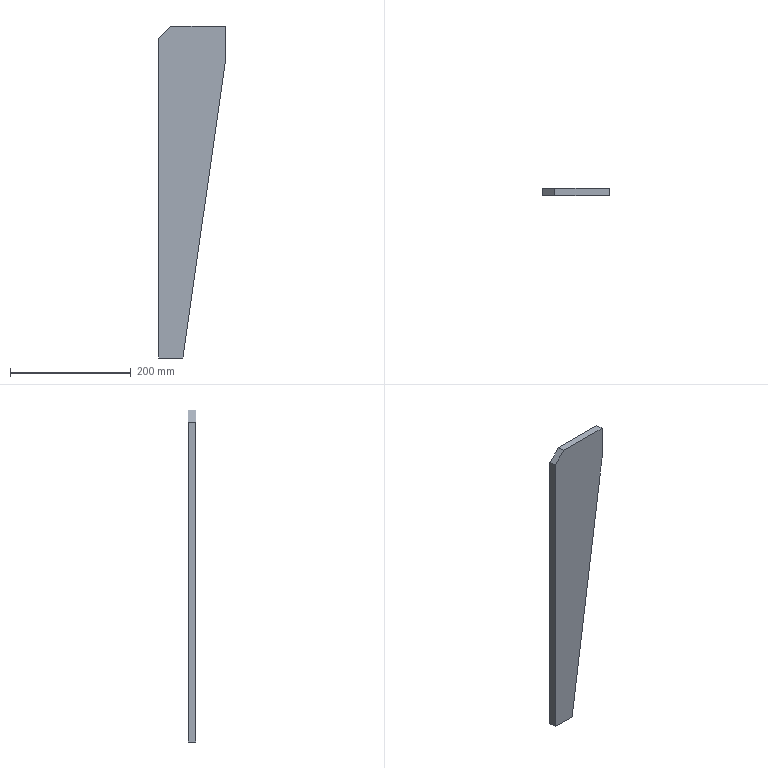Part | SolidWorks | features Chamfer 1, Extrusion 1 | 1 solid | 8 faces | box 110 x 12 x 550 mm | volume 517800 mm3 | plane 8
STEP:
#1=CARTESIAN_POINT('',(0.,6.,0.));
#2=VERTEX_POINT('',#1);
#3=CARTESIAN_POINT('',(90.,6.,0.));
#4=VERTEX_POINT('',#3);
#5=CARTESIAN_POINT('',(-20.,6.,0.));
#6=DIRECTION('',(1.,0.,0.));
#7=VECTOR('',#6,1000.);
#8=LINE('',#5,#7);
#9=EDGE_CURVE('',#2,#4,#8,.T.);
#10=ORIENTED_EDGE('',*,*,#9,.F.);
#11=CARTESIAN_POINT('',(0.,-6.,0.));
#12=VERTEX_POINT('',#11);
#13=CARTESIAN_POINT('',(0.,6.,0.));
#14=DIRECTION('',(0.,-1.,0.));
#15=VECTOR('',#14,1000.);
#16=LINE('',#13,#15);
#17=EDGE_CURVE('',#2,#12,#16,.T.);
#18=ORIENTED_EDGE('',*,*,#17,.T.);
#19=CARTESIAN_POINT('',(90.,-6.,0.));
#20=VERTEX_POINT('',#19);
#21=CARTESIAN_POINT('',(90.,-6.,0.));
#22=DIRECTION('',(1.,0.,0.));
#23=VECTOR('',#22,1000.);
#24=LINE('',#21,#23);
#25=EDGE_CURVE('',#12,#20,#24,.T.);
#26=ORIENTED_EDGE('',*,*,#25,.T.);
#27=CARTESIAN_POINT('',(90.,6.,0.));
#28=DIRECTION('',(0.,-1.,0.));
#29=VECTOR('',#28,1000.);
#30=LINE('',#27,#29);
#31=EDGE_CURVE('',#4,#20,#30,.T.);
#32=ORIENTED_EDGE('',*,*,#31,.F.);
#33=EDGE_LOOP('',(#10,#18,#26,#32));
#34=FACE_OUTER_BOUND('',#33,.T.);
#35=CARTESIAN_POINT('',(90.,6.,0.));
#36=DIRECTION('',(0.,0.,-1.));
#37=DIRECTION('',(-1.,0.,0.));
#38=AXIS2_PLACEMENT_3D('',#35,#36,#37);
#39=PLANE('',#38);
#40=ADVANCED_FACE('',(#34),#39,.F.);
#41=CARTESIAN_POINT('',(90.,-6.,-60.));
#42=VERTEX_POINT('',#41);
#43=CARTESIAN_POINT('',(90.,-6.,-60.));
#44=DIRECTION('',(0.,0.,-1.));
#45=VECTOR('',#44,1000.);
#46=LINE('',#43,#45);
#47=EDGE_CURVE('',#20,#42,#46,.T.);
#48=ORIENTED_EDGE('',*,*,#47,.T.);
#49=CARTESIAN_POINT('',(90.,6.,-60.));
#50=VERTEX_POINT('',#49);
#51=CARTESIAN_POINT('',(90.,6.,-60.));
#52=DIRECTION('',(0.,-1.,0.));
#53=VECTOR('',#52,1000.);
#54=LINE('',#51,#53);
#55=EDGE_CURVE('',#50,#42,#54,.T.);
#56=ORIENTED_EDGE('',*,*,#55,.F.);
#57=CARTESIAN_POINT('',(90.,6.,-60.));
#58=DIRECTION('',(0.,0.,-1.));
#59=VECTOR('',#58,1000.);
#60=LINE('',#57,#59);
#61=EDGE_CURVE('',#4,#50,#60,.T.);
#62=ORIENTED_EDGE('',*,*,#61,.F.);
#63=ORIENTED_EDGE('',*,*,#31,.T.);
#64=EDGE_LOOP('',(#48,#56,#62,#63));
#65=FACE_OUTER_BOUND('',#64,.T.);
#66=CARTESIAN_POINT('',(90.,6.,-60.));
#67=DIRECTION('',(-1.,0.,0.));
#68=DIRECTION('',(0.,0.,1.));
#69=AXIS2_PLACEMENT_3D('',#66,#67,#68);
#70=PLANE('',#69);
#71=ADVANCED_FACE('',(#65),#70,.F.);
#72=CARTESIAN_POINT('',(20.,-6.,-550.));
#73=VERTEX_POINT('',#72);
#74=CARTESIAN_POINT('',(20.,-6.,-550.));
#75=DIRECTION('',(-0.1414,0.,-0.9899));
#76=VECTOR('',#75,1000.);
#77=LINE('',#74,#76);
#78=EDGE_CURVE('',#42,#73,#77,.T.);
#79=ORIENTED_EDGE('',*,*,#78,.T.);
#80=CARTESIAN_POINT('',(20.,6.,-550.));
#81=VERTEX_POINT('',#80);
#82=CARTESIAN_POINT('',(20.,6.,-550.));
#83=DIRECTION('',(0.,-1.,0.));
#84=VECTOR('',#83,1000.);
#85=LINE('',#82,#84);
#86=EDGE_CURVE('',#81,#73,#85,.T.);
#87=ORIENTED_EDGE('',*,*,#86,.F.);
#88=CARTESIAN_POINT('',(20.,6.,-550.));
#89=DIRECTION('',(-0.1414,0.,-0.9899));
#90=VECTOR('',#89,1000.);
#91=LINE('',#88,#90);
#92=EDGE_CURVE('',#50,#81,#91,.T.);
#93=ORIENTED_EDGE('',*,*,#92,.F.);
#94=ORIENTED_EDGE('',*,*,#55,.T.);
#95=EDGE_LOOP('',(#79,#87,#93,#94));
#96=FACE_OUTER_BOUND('',#95,.T.);
#97=CARTESIAN_POINT('',(20.,6.,-550.));
#98=DIRECTION('',(-0.9899,0.,0.1414));
#99=DIRECTION('',(0.1414,0.,0.9899));
#100=AXIS2_PLACEMENT_3D('',#97,#98,#99);
#101=PLANE('',#100);
#102=ADVANCED_FACE('',(#96),#101,.F.);
#103=CARTESIAN_POINT('',(-20.,-6.,-550.));
#104=VERTEX_POINT('',#103);
#105=CARTESIAN_POINT('',(-20.,-6.,-550.));
#106=DIRECTION('',(-1.,0.,0.));
#107=VECTOR('',#106,1000.);
#108=LINE('',#105,#107);
#109=EDGE_CURVE('',#73,#104,#108,.T.);
#110=ORIENTED_EDGE('',*,*,#109,.T.);
#111=CARTESIAN_POINT('',(-20.,6.,-550.));
#112=VERTEX_POINT('',#111);
#113=CARTESIAN_POINT('',(-20.,6.,-550.));
#114=DIRECTION('',(0.,-1.,0.));
#115=VECTOR('',#114,1000.);
#116=LINE('',#113,#115);
#117=EDGE_CURVE('',#112,#104,#116,.T.);
#118=ORIENTED_EDGE('',*,*,#117,.F.);
#119=CARTESIAN_POINT('',(-20.,6.,-550.));
#120=DIRECTION('',(-1.,0.,0.));
#121=VECTOR('',#120,1000.);
#122=LINE('',#119,#121);
#123=EDGE_CURVE('',#81,#112,#122,.T.);
#124=ORIENTED_EDGE('',*,*,#123,.F.);
#125=ORIENTED_EDGE('',*,*,#86,.T.);
#126=EDGE_LOOP('',(#110,#118,#124,#125));
#127=FACE_OUTER_BOUND('',#126,.T.);
#128=CARTESIAN_POINT('',(-20.,6.,-550.));
#129=DIRECTION('',(0.,0.,1.));
#130=DIRECTION('',(1.,0.,0.));
#131=AXIS2_PLACEMENT_3D('',#128,#129,#130);
#132=PLANE('',#131);
#133=ADVANCED_FACE('',(#127),#132,.F.);
#134=CARTESIAN_POINT('',(-20.,-6.,-20.));
#135=VERTEX_POINT('',#134);
#136=CARTESIAN_POINT('',(-20.,-6.,-20.));
#137=DIRECTION('',(0.,0.,1.));
#138=VECTOR('',#137,1000.);
#139=LINE('',#136,#138);
#140=EDGE_CURVE('',#104,#135,#139,.T.);
#141=ORIENTED_EDGE('',*,*,#140,.T.);
#142=CARTESIAN_POINT('',(-20.,6.,-20.));
#143=VERTEX_POINT('',#142);
#144=CARTESIAN_POINT('',(-20.,6.,-20.));
#145=DIRECTION('',(0.,1.,0.));
#146=VECTOR('',#145,1000.);
#147=LINE('',#144,#146);
#148=EDGE_CURVE('',#135,#143,#147,.T.);
#149=ORIENTED_EDGE('',*,*,#148,.T.);
#150=CARTESIAN_POINT('',(-20.,6.,-20.));
#151=DIRECTION('',(0.,0.,1.));
#152=VECTOR('',#151,1000.);
#153=LINE('',#150,#152);
#154=EDGE_CURVE('',#112,#143,#153,.T.);
#155=ORIENTED_EDGE('',*,*,#154,.F.);
#156=ORIENTED_EDGE('',*,*,#117,.T.);
#157=EDGE_LOOP('',(#141,#149,#155,#156));
#158=FACE_OUTER_BOUND('',#157,.T.);
#159=CARTESIAN_POINT('',(-20.,6.,-20.));
#160=DIRECTION('',(1.,0.,0.));
#161=DIRECTION('',(0.,0.,-1.));
#162=AXIS2_PLACEMENT_3D('',#159,#160,#161);
#163=PLANE('',#162);
#164=ADVANCED_FACE('',(#158),#163,.F.);
#165=ORIENTED_EDGE('',*,*,#154,.T.);
#166=CARTESIAN_POINT('',(0.,6.,0.));
#167=DIRECTION('',(0.7071,0.,0.7071));
#168=VECTOR('',#167,1000.);
#169=LINE('',#166,#168);
#170=EDGE_CURVE('',#143,#2,#169,.T.);
#171=ORIENTED_EDGE('',*,*,#170,.T.);
#172=ORIENTED_EDGE('',*,*,#9,.T.);
#173=ORIENTED_EDGE('',*,*,#61,.T.);
#174=ORIENTED_EDGE('',*,*,#92,.T.);
#175=ORIENTED_EDGE('',*,*,#123,.T.);
#176=EDGE_LOOP('',(#165,#171,#172,#173,#174,#175));
#177=FACE_OUTER_BOUND('',#176,.T.);
#178=CARTESIAN_POINT('',(0.,6.,0.));
#179=DIRECTION('',(0.,-1.,0.));
#180=DIRECTION('',(0.,0.,-1.));
#181=AXIS2_PLACEMENT_3D('',#178,#179,#180);
#182=PLANE('',#181);
#183=ADVANCED_FACE('',(#177),#182,.F.);
#184=ORIENTED_EDGE('',*,*,#25,.F.);
#185=CARTESIAN_POINT('',(0.,-6.,0.));
#186=DIRECTION('',(-0.7071,0.,-0.7071));
#187=VECTOR('',#186,1000.);
#188=LINE('',#185,#187);
#189=EDGE_CURVE('',#12,#135,#188,.T.);
#190=ORIENTED_EDGE('',*,*,#189,.T.);
#191=ORIENTED_EDGE('',*,*,#140,.F.);
#192=ORIENTED_EDGE('',*,*,#109,.F.);
#193=ORIENTED_EDGE('',*,*,#78,.F.);
#194=ORIENTED_EDGE('',*,*,#47,.F.);
#195=EDGE_LOOP('',(#184,#190,#191,#192,#193,#194));
#196=FACE_OUTER_BOUND('',#195,.T.);
#197=CARTESIAN_POINT('',(0.,-6.,0.));
#198=DIRECTION('',(0.,-1.,0.));
#199=DIRECTION('',(0.,0.,-1.));
#200=AXIS2_PLACEMENT_3D('',#197,#198,#199);
#201=PLANE('',#200);
#202=ADVANCED_FACE('',(#196),#201,.T.);
#203=ORIENTED_EDGE('',*,*,#170,.F.);
#204=ORIENTED_EDGE('',*,*,#148,.F.);
#205=ORIENTED_EDGE('',*,*,#189,.F.);
#206=ORIENTED_EDGE('',*,*,#17,.F.);
#207=EDGE_LOOP('',(#203,#204,#205,#206));
#208=FACE_OUTER_BOUND('',#207,.T.);
#209=CARTESIAN_POINT('',(0.,6.,0.));
#210=DIRECTION('',(0.7071,0.,-0.7071));
#211=DIRECTION('',(0.,-1.,0.));
#212=AXIS2_PLACEMENT_3D('',#209,#210,#211);
#213=PLANE('',#212);
#214=ADVANCED_FACE('',(#208),#213,.F.);
#215=CLOSED_SHELL('',(#40,#71,#102,#133,#164,#183,#202,#214));
#216=MANIFOLD_SOLID_BREP('',#215);
#217=CARTESIAN_POINT('',(0.,0.,0.));
#218=DIRECTION('',(0.,0.,1.));
#219=DIRECTION('',(1.,0.,0.));
#220=AXIS2_PLACEMENT_3D('',#217,#218,#219);
#221=(LENGTH_UNIT()NAMED_UNIT(*)SI_UNIT(.MILLI.,.METRE.));
#222=UNCERTAINTY_MEASURE_WITH_UNIT(LENGTH_MEASURE(0.00001),#221,'','');
#223=(NAMED_UNIT(*)PLANE_ANGLE_UNIT()SI_UNIT($,.RADIAN.));
#224=(NAMED_UNIT(*)SI_UNIT($,.STERADIAN.)SOLID_ANGLE_UNIT());
#225=(GEOMETRIC_REPRESENTATION_CONTEXT(3)GLOBAL_UNCERTAINTY_ASSIGNED_CONTEXT((#222))GLOBAL_UNIT_ASSIGNED_CONTEXT((#221,#223,#224))REPRESENTATION_CONTEXT('',''));
#226=ADVANCED_BREP_SHAPE_REPRESENTATION('',(#216,#220),#225);